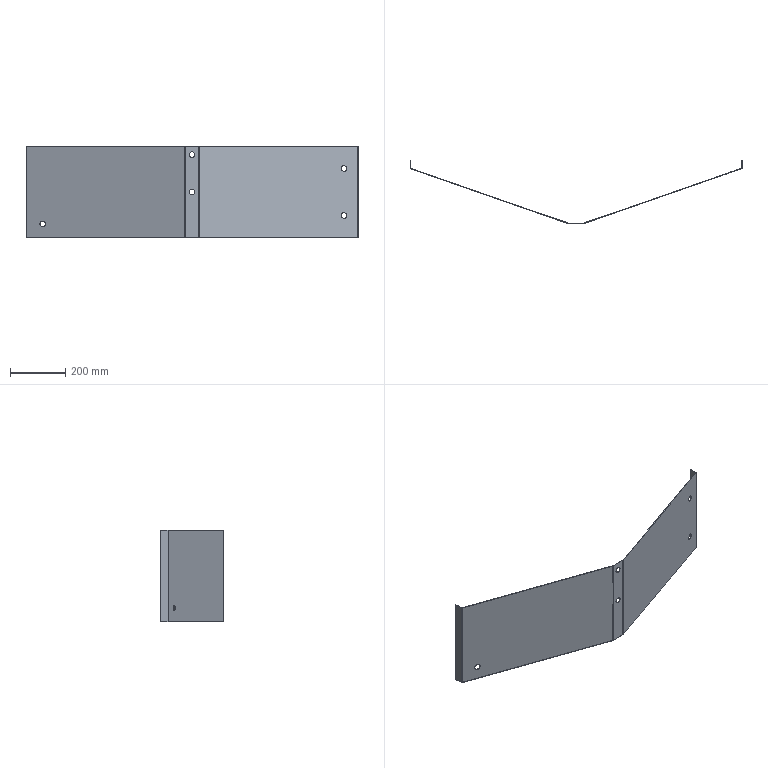Part | SolidWorks | features ICE 4, FlatPattern 1, SMBaseFlange 1, SheetMetal 1 | 1 solid | 48 faces | box 1200 x 230 x 330 mm | volume 522694 mm3 | plane 30 | cylinder 18 | commonest cylinder face diameters 20 x10 2 x4 4.4 x4
STEP:
#1=CARTESIAN_POINT('',(60.329,-19.714,40.));
#2=VERTEX_POINT('',#1);
#3=CARTESIAN_POINT('',(60.329,-19.714,60.));
#4=VERTEX_POINT('',#3);
#5=CARTESIAN_POINT('',(60.329,-19.714,40.));
#6=CARTESIAN_POINT('',(40.329,-12.757,40.));
#7=CARTESIAN_POINT('',(40.329,-12.757,60.));
#8=CARTESIAN_POINT('',(60.329,-19.714,60.));
#9=(BOUNDED_CURVE()B_SPLINE_CURVE(3,(#5,#6,#7,#8),.UNSPECIFIED.,.F.,.F.)B_SPLINE_CURVE_WITH_KNOTS((4,4),(1.571,4.712),.UNSPECIFIED.)CURVE()GEOMETRIC_REPRESENTATION_ITEM()RATIONAL_B_SPLINE_CURVE((1.,0.3333,0.3333,1.))REPRESENTATION_ITEM(''));
#10=EDGE_CURVE('',#2,#4,#9,.T.);
#11=ORIENTED_EDGE('',*,*,#10,.T.);
#12=CARTESIAN_POINT('',(60.329,-20.984,60.));
#13=VERTEX_POINT('',#12);
#14=CARTESIAN_POINT('',(60.329,30.,60.));
#15=DIRECTION('',(0.,-1.,0.));
#16=VECTOR('',#15,1000.);
#17=LINE('',#14,#16);
#18=EDGE_CURVE('',#4,#13,#17,.T.);
#19=ORIENTED_EDGE('',*,*,#18,.T.);
#20=CARTESIAN_POINT('',(60.329,-20.984,40.));
#21=VERTEX_POINT('',#20);
#22=CARTESIAN_POINT('',(60.329,-20.984,40.));
#23=CARTESIAN_POINT('',(40.329,-14.028,40.));
#24=CARTESIAN_POINT('',(40.329,-14.028,60.));
#25=CARTESIAN_POINT('',(60.329,-20.984,60.));
#26=(BOUNDED_CURVE()B_SPLINE_CURVE(3,(#22,#23,#24,#25),.UNSPECIFIED.,.F.,.F.)B_SPLINE_CURVE_WITH_KNOTS((4,4),(1.571,4.712),.UNSPECIFIED.)CURVE()GEOMETRIC_REPRESENTATION_ITEM()RATIONAL_B_SPLINE_CURVE((1.,0.3333,0.3333,1.))REPRESENTATION_ITEM(''));
#27=EDGE_CURVE('',#21,#13,#26,.T.);
#28=ORIENTED_EDGE('',*,*,#27,.F.);
#29=CARTESIAN_POINT('',(60.329,30.,40.));
#30=DIRECTION('',(0.,-1.,0.));
#31=VECTOR('',#30,1000.);
#32=LINE('',#29,#31);
#33=EDGE_CURVE('',#2,#21,#32,.T.);
#34=ORIENTED_EDGE('',*,*,#33,.F.);
#35=EDGE_LOOP('',(#11,#19,#28,#34));
#36=FACE_OUTER_BOUND('',#35,.T.);
#37=CARTESIAN_POINT('',(60.329,30.,50.));
#38=DIRECTION('',(0.,-1.,0.));
#39=DIRECTION('',(0.,0.,-1.));
#40=AXIS2_PLACEMENT_3D('',#37,#38,#39);
#41=CYLINDRICAL_SURFACE('',#40,10.);
#42=ADVANCED_FACE('',(#36),#41,.F.);
#43=CARTESIAN_POINT('',(1149.665,-16.237,240.));
#44=VERTEX_POINT('',#43);
#45=CARTESIAN_POINT('',(1149.665,-16.237,260.));
#46=VERTEX_POINT('',#45);
#47=CARTESIAN_POINT('',(1149.665,-16.237,240.));
#48=CARTESIAN_POINT('',(1129.665,-23.194,240.));
#49=CARTESIAN_POINT('',(1129.665,-23.194,260.));
#50=CARTESIAN_POINT('',(1149.665,-16.237,260.));
#51=(BOUNDED_CURVE()B_SPLINE_CURVE(3,(#47,#48,#49,#50),.UNSPECIFIED.,.F.,.F.)B_SPLINE_CURVE_WITH_KNOTS((4,4),(4.712,7.854),.UNSPECIFIED.)CURVE()GEOMETRIC_REPRESENTATION_ITEM()RATIONAL_B_SPLINE_CURVE((1.,0.3333,0.3333,1.))REPRESENTATION_ITEM(''));
#52=EDGE_CURVE('',#44,#46,#51,.T.);
#53=ORIENTED_EDGE('',*,*,#52,.T.);
#54=CARTESIAN_POINT('',(1149.665,-17.508,260.));
#55=VERTEX_POINT('',#54);
#56=CARTESIAN_POINT('',(1149.665,30.,260.));
#57=DIRECTION('',(0.,-1.,0.));
#58=VECTOR('',#57,1000.);
#59=LINE('',#56,#58);
#60=EDGE_CURVE('',#46,#55,#59,.T.);
#61=ORIENTED_EDGE('',*,*,#60,.T.);
#62=CARTESIAN_POINT('',(1149.665,-17.508,240.));
#63=VERTEX_POINT('',#62);
#64=CARTESIAN_POINT('',(1149.665,-17.508,240.));
#65=CARTESIAN_POINT('',(1129.665,-24.464,240.));
#66=CARTESIAN_POINT('',(1129.665,-24.464,260.));
#67=CARTESIAN_POINT('',(1149.665,-17.508,260.));
#68=(BOUNDED_CURVE()B_SPLINE_CURVE(3,(#64,#65,#66,#67),.UNSPECIFIED.,.F.,.F.)B_SPLINE_CURVE_WITH_KNOTS((4,4),(4.712,7.854),.UNSPECIFIED.)CURVE()GEOMETRIC_REPRESENTATION_ITEM()RATIONAL_B_SPLINE_CURVE((1.,0.3333,0.3333,1.))REPRESENTATION_ITEM(''));
#69=EDGE_CURVE('',#63,#55,#68,.T.);
#70=ORIENTED_EDGE('',*,*,#69,.F.);
#71=CARTESIAN_POINT('',(1149.665,30.,240.));
#72=DIRECTION('',(0.,-1.,0.));
#73=VECTOR('',#72,1000.);
#74=LINE('',#71,#73);
#75=EDGE_CURVE('',#44,#63,#74,.T.);
#76=ORIENTED_EDGE('',*,*,#75,.F.);
#77=EDGE_LOOP('',(#53,#61,#70,#76));
#78=FACE_OUTER_BOUND('',#77,.T.);
#79=CARTESIAN_POINT('',(1149.665,30.,250.));
#80=DIRECTION('',(0.,-1.,0.));
#81=DIRECTION('',(0.,0.,-1.));
#82=AXIS2_PLACEMENT_3D('',#79,#80,#81);
#83=CYLINDRICAL_SURFACE('',#82,10.);
#84=ADVANCED_FACE('',(#78),#83,.F.);
#85=CARTESIAN_POINT('',(1149.665,-16.237,70.));
#86=VERTEX_POINT('',#85);
#87=CARTESIAN_POINT('',(1149.665,-16.237,90.));
#88=VERTEX_POINT('',#87);
#89=CARTESIAN_POINT('',(1149.665,-16.237,70.));
#90=CARTESIAN_POINT('',(1129.665,-23.194,70.));
#91=CARTESIAN_POINT('',(1129.665,-23.194,90.));
#92=CARTESIAN_POINT('',(1149.665,-16.237,90.));
#93=(BOUNDED_CURVE()B_SPLINE_CURVE(3,(#89,#90,#91,#92),.UNSPECIFIED.,.F.,.F.)B_SPLINE_CURVE_WITH_KNOTS((4,4),(4.712,7.854),.UNSPECIFIED.)CURVE()GEOMETRIC_REPRESENTATION_ITEM()RATIONAL_B_SPLINE_CURVE((1.,0.3333,0.3333,1.))REPRESENTATION_ITEM(''));
#94=EDGE_CURVE('',#86,#88,#93,.T.);
#95=ORIENTED_EDGE('',*,*,#94,.T.);
#96=CARTESIAN_POINT('',(1149.665,-17.508,90.));
#97=VERTEX_POINT('',#96);
#98=CARTESIAN_POINT('',(1149.665,30.,90.));
#99=DIRECTION('',(0.,-1.,0.));
#100=VECTOR('',#99,1000.);
#101=LINE('',#98,#100);
#102=EDGE_CURVE('',#88,#97,#101,.T.);
#103=ORIENTED_EDGE('',*,*,#102,.T.);
#104=CARTESIAN_POINT('',(1149.665,-17.508,70.));
#105=VERTEX_POINT('',#104);
#106=CARTESIAN_POINT('',(1149.665,-17.508,70.));
#107=CARTESIAN_POINT('',(1129.665,-24.464,70.));
#108=CARTESIAN_POINT('',(1129.665,-24.464,90.));
#109=CARTESIAN_POINT('',(1149.665,-17.508,90.));
#110=(BOUNDED_CURVE()B_SPLINE_CURVE(3,(#106,#107,#108,#109),.UNSPECIFIED.,.F.,.F.)B_SPLINE_CURVE_WITH_KNOTS((4,4),(4.712,7.854),.UNSPECIFIED.)CURVE()GEOMETRIC_REPRESENTATION_ITEM()RATIONAL_B_SPLINE_CURVE((1.,0.3333,0.3333,1.))REPRESENTATION_ITEM(''));
#111=EDGE_CURVE('',#105,#97,#110,.T.);
#112=ORIENTED_EDGE('',*,*,#111,.F.);
#113=CARTESIAN_POINT('',(1149.665,30.,70.));
#114=DIRECTION('',(0.,-1.,0.));
#115=VECTOR('',#114,1000.);
#116=LINE('',#113,#115);
#117=EDGE_CURVE('',#86,#105,#116,.T.);
#118=ORIENTED_EDGE('',*,*,#117,.F.);
#119=EDGE_LOOP('',(#95,#103,#112,#118));
#120=FACE_OUTER_BOUND('',#119,.T.);
#121=CARTESIAN_POINT('',(1149.665,30.,80.));
#122=DIRECTION('',(0.,-1.,0.));
#123=DIRECTION('',(0.,0.,-1.));
#124=AXIS2_PLACEMENT_3D('',#121,#122,#123);
#125=CYLINDRICAL_SURFACE('',#124,10.);
#126=ADVANCED_FACE('',(#120),#125,.F.);
#127=CARTESIAN_POINT('',(600.,-200.,155.));
#128=VERTEX_POINT('',#127);
#129=CARTESIAN_POINT('',(600.,-200.,175.));
#130=VERTEX_POINT('',#129);
#131=CARTESIAN_POINT('',(600.,-200.,165.));
#132=DIRECTION('',(0.,1.,0.));
#133=DIRECTION('',(0.,0.,1.));
#134=AXIS2_PLACEMENT_3D('',#131,#132,#133);
#135=CIRCLE('',#134,10.);
#136=EDGE_CURVE('',#128,#130,#135,.T.);
#137=ORIENTED_EDGE('',*,*,#136,.F.);
#138=CARTESIAN_POINT('',(600.,-198.8,155.));
#139=VERTEX_POINT('',#138);
#140=CARTESIAN_POINT('',(600.,-208.8,155.));
#141=DIRECTION('',(0.,1.,0.));
#142=VECTOR('',#141,1000.);
#143=LINE('',#140,#142);
#144=EDGE_CURVE('',#128,#139,#143,.T.);
#145=ORIENTED_EDGE('',*,*,#144,.T.);
#146=CARTESIAN_POINT('',(600.,-198.8,175.));
#147=VERTEX_POINT('',#146);
#148=CARTESIAN_POINT('',(600.,-198.8,165.));
#149=DIRECTION('',(0.,1.,0.));
#150=DIRECTION('',(0.,0.,1.));
#151=AXIS2_PLACEMENT_3D('',#148,#149,#150);
#152=CIRCLE('',#151,10.);
#153=EDGE_CURVE('',#139,#147,#152,.T.);
#154=ORIENTED_EDGE('',*,*,#153,.T.);
#155=CARTESIAN_POINT('',(600.,-208.8,175.));
#156=DIRECTION('',(0.,1.,0.));
#157=VECTOR('',#156,1000.);
#158=LINE('',#155,#157);
#159=EDGE_CURVE('',#130,#147,#158,.T.);
#160=ORIENTED_EDGE('',*,*,#159,.F.);
#161=EDGE_LOOP('',(#137,#145,#154,#160));
#162=FACE_OUTER_BOUND('',#161,.T.);
#163=CARTESIAN_POINT('',(600.,-208.8,165.));
#164=DIRECTION('',(0.,1.,0.));
#165=DIRECTION('',(0.,0.,1.));
#166=AXIS2_PLACEMENT_3D('',#163,#164,#165);
#167=CYLINDRICAL_SURFACE('',#166,10.);
#168=ADVANCED_FACE('',(#162),#167,.F.);
#169=CARTESIAN_POINT('',(600.,-200.,290.));
#170=VERTEX_POINT('',#169);
#171=CARTESIAN_POINT('',(600.,-200.,310.));
#172=VERTEX_POINT('',#171);
#173=CARTESIAN_POINT('',(600.,-200.,300.));
#174=DIRECTION('',(0.,1.,0.));
#175=DIRECTION('',(0.,0.,1.));
#176=AXIS2_PLACEMENT_3D('',#173,#174,#175);
#177=CIRCLE('',#176,10.);
#178=EDGE_CURVE('',#170,#172,#177,.T.);
#179=ORIENTED_EDGE('',*,*,#178,.F.);
#180=CARTESIAN_POINT('',(600.,-198.8,290.));
#181=VERTEX_POINT('',#180);
#182=CARTESIAN_POINT('',(600.,-208.8,290.));
#183=DIRECTION('',(0.,1.,0.));
#184=VECTOR('',#183,1000.);
#185=LINE('',#182,#184);
#186=EDGE_CURVE('',#170,#181,#185,.T.);
#187=ORIENTED_EDGE('',*,*,#186,.T.);
#188=CARTESIAN_POINT('',(600.,-198.8,310.));
#189=VERTEX_POINT('',#188);
#190=CARTESIAN_POINT('',(600.,-198.8,300.));
#191=DIRECTION('',(0.,1.,0.));
#192=DIRECTION('',(0.,0.,1.));
#193=AXIS2_PLACEMENT_3D('',#190,#191,#192);
#194=CIRCLE('',#193,10.);
#195=EDGE_CURVE('',#181,#189,#194,.T.);
#196=ORIENTED_EDGE('',*,*,#195,.T.);
#197=CARTESIAN_POINT('',(600.,-208.8,310.));
#198=DIRECTION('',(0.,1.,0.));
#199=VECTOR('',#198,1000.);
#200=LINE('',#197,#199);
#201=EDGE_CURVE('',#172,#189,#200,.T.);
#202=ORIENTED_EDGE('',*,*,#201,.F.);
#203=EDGE_LOOP('',(#179,#187,#196,#202));
#204=FACE_OUTER_BOUND('',#203,.T.);
#205=CARTESIAN_POINT('',(600.,-208.8,300.));
#206=DIRECTION('',(0.,1.,0.));
#207=DIRECTION('',(0.,0.,1.));
#208=AXIS2_PLACEMENT_3D('',#205,#206,#207);
#209=CYLINDRICAL_SURFACE('',#208,10.);
#210=ADVANCED_FACE('',(#204),#209,.F.);
#211=CARTESIAN_POINT('',(0.,1.564,330.));
#212=VERTEX_POINT('',#211);
#213=CARTESIAN_POINT('',(1.2,1.564,330.));
#214=VERTEX_POINT('',#213);
#215=CARTESIAN_POINT('',(0.,1.564,330.));
#216=DIRECTION('',(1.,0.,0.));
#217=VECTOR('',#216,1000.);
#218=LINE('',#215,#217);
#219=EDGE_CURVE('',#212,#214,#218,.T.);
#220=ORIENTED_EDGE('',*,*,#219,.F.);
#221=CARTESIAN_POINT('',(1.477,-0.5138,330.));
#222=VERTEX_POINT('',#221);
#223=CARTESIAN_POINT('',(2.2,1.564,330.));
#224=DIRECTION('',(0.,0.,1.));
#225=DIRECTION('',(-1.,0.,0.));
#226=AXIS2_PLACEMENT_3D('',#223,#224,#225);
#227=CIRCLE('',#226,2.2);
#228=EDGE_CURVE('',#212,#222,#227,.T.);
#229=ORIENTED_EDGE('',*,*,#228,.T.);
#230=CARTESIAN_POINT('',(1.871,0.6196,330.));
#231=VERTEX_POINT('',#230);
#232=CARTESIAN_POINT('',(1.871,0.6196,330.));
#233=DIRECTION('',(-0.3285,-0.9445,0.));
#234=VECTOR('',#233,1000.);
#235=LINE('',#232,#234);
#236=EDGE_CURVE('',#231,#222,#235,.T.);
#237=ORIENTED_EDGE('',*,*,#236,.F.);
#238=CARTESIAN_POINT('',(2.2,1.564,330.));
#239=DIRECTION('',(0.,0.,1.));
#240=DIRECTION('',(1.,0.,0.));
#241=AXIS2_PLACEMENT_3D('',#238,#239,#240);
#242=CIRCLE('',#241,1.);
#243=EDGE_CURVE('',#214,#231,#242,.T.);
#244=ORIENTED_EDGE('',*,*,#243,.F.);
#245=EDGE_LOOP('',(#220,#229,#237,#244));
#246=FACE_OUTER_BOUND('',#245,.T.);
#247=CARTESIAN_POINT('',(0.,1.564,330.));
#248=DIRECTION('',(0.,0.,1.));
#249=DIRECTION('',(1.,0.,0.));
#250=AXIS2_PLACEMENT_3D('',#247,#248,#249);
#251=PLANE('',#250);
#252=ADVANCED_FACE('',(#246),#251,.T.);
#253=CARTESIAN_POINT('',(0.,30.,330.));
#254=VERTEX_POINT('',#253);
#255=CARTESIAN_POINT('',(0.,0.,330.));
#256=DIRECTION('',(0.,-1.,0.));
#257=VECTOR('',#256,1000.);
#258=LINE('',#255,#257);
#259=EDGE_CURVE('',#254,#212,#258,.T.);
#260=ORIENTED_EDGE('',*,*,#259,.T.);
#261=ORIENTED_EDGE('',*,*,#219,.T.);
#262=CARTESIAN_POINT('',(1.2,30.,330.));
#263=VERTEX_POINT('',#262);
#264=CARTESIAN_POINT('',(1.2,0.,330.));
#265=DIRECTION('',(0.,-1.,0.));
#266=VECTOR('',#265,1000.);
#267=LINE('',#264,#266);
#268=EDGE_CURVE('',#263,#214,#267,.T.);
#269=ORIENTED_EDGE('',*,*,#268,.F.);
#270=CARTESIAN_POINT('',(0.,30.,330.));
#271=DIRECTION('',(1.,0.,0.));
#272=VECTOR('',#271,1000.);
#273=LINE('',#270,#272);
#274=EDGE_CURVE('',#254,#263,#273,.T.);
#275=ORIENTED_EDGE('',*,*,#274,.F.);
#276=EDGE_LOOP('',(#260,#261,#269,#275));
#277=FACE_OUTER_BOUND('',#276,.T.);
#278=CARTESIAN_POINT('',(1.871,0.6196,330.));
#279=DIRECTION('',(0.,0.,1.));
#280=DIRECTION('',(1.,0.,0.));
#281=AXIS2_PLACEMENT_3D('',#278,#279,#280);
#282=PLANE('',#281);
#283=ADVANCED_FACE('',(#277),#282,.T.);
#284=CARTESIAN_POINT('',(1.477,-0.5138,0.));
#285=VERTEX_POINT('',#284);
#286=CARTESIAN_POINT('',(1.871,0.6196,0.));
#287=VERTEX_POINT('',#286);
#288=CARTESIAN_POINT('',(1.477,-0.5138,0.));
#289=DIRECTION('',(0.3285,0.9445,0.));
#290=VECTOR('',#289,1000.);
#291=LINE('',#288,#290);
#292=EDGE_CURVE('',#285,#287,#291,.T.);
#293=ORIENTED_EDGE('',*,*,#292,.F.);
#294=CARTESIAN_POINT('',(0.,1.564,0.));
#295=VERTEX_POINT('',#294);
#296=CARTESIAN_POINT('',(2.2,1.564,0.));
#297=DIRECTION('',(0.,0.,1.));
#298=DIRECTION('',(-1.,0.,0.));
#299=AXIS2_PLACEMENT_3D('',#296,#297,#298);
#300=CIRCLE('',#299,2.2);
#301=EDGE_CURVE('',#295,#285,#300,.T.);
#302=ORIENTED_EDGE('',*,*,#301,.F.);
#303=CARTESIAN_POINT('',(1.2,1.564,0.));
#304=VERTEX_POINT('',#303);
#305=CARTESIAN_POINT('',(1.2,1.564,0.));
#306=DIRECTION('',(-1.,0.,0.));
#307=VECTOR('',#306,1000.);
#308=LINE('',#305,#307);
#309=EDGE_CURVE('',#304,#295,#308,.T.);
#310=ORIENTED_EDGE('',*,*,#309,.F.);
#311=CARTESIAN_POINT('',(2.2,1.564,0.));
#312=DIRECTION('',(0.,0.,1.));
#313=DIRECTION('',(1.,0.,0.));
#314=AXIS2_PLACEMENT_3D('',#311,#312,#313);
#315=CIRCLE('',#314,1.);
#316=EDGE_CURVE('',#304,#287,#315,.T.);
#317=ORIENTED_EDGE('',*,*,#316,.T.);
#318=EDGE_LOOP('',(#293,#302,#310,#317));
#319=FACE_OUTER_BOUND('',#318,.T.);
#320=CARTESIAN_POINT('',(1.477,-0.5138,0.));
#321=DIRECTION('',(0.,0.,-1.));
#322=DIRECTION('',(-1.,0.,0.));
#323=AXIS2_PLACEMENT_3D('',#320,#321,#322);
#324=PLANE('',#323);
#325=ADVANCED_FACE('',(#319),#324,.T.);
#326=CARTESIAN_POINT('',(574.649,-199.878,0.));
#327=VERTEX_POINT('',#326);
#328=CARTESIAN_POINT('',(0.,0.,0.));
#329=DIRECTION('',(0.9445,-0.3285,0.));
#330=VECTOR('',#329,1000.);
#331=LINE('',#328,#330);
#332=EDGE_CURVE('',#285,#327,#331,.T.);
#333=ORIENTED_EDGE('',*,*,#332,.F.);
#334=ORIENTED_EDGE('',*,*,#292,.T.);
#335=CARTESIAN_POINT('',(575.043,-198.744,0.));
#336=VERTEX_POINT('',#335);
#337=CARTESIAN_POINT('',(0.3942,1.133,0.));
#338=DIRECTION('',(0.9445,-0.3285,0.));
#339=VECTOR('',#338,1000.);
#340=LINE('',#337,#339);
#341=EDGE_CURVE('',#287,#336,#340,.T.);
#342=ORIENTED_EDGE('',*,*,#341,.T.);
#343=CARTESIAN_POINT('',(575.043,-198.744,0.));
#344=DIRECTION('',(-0.3285,-0.9445,0.));
#345=VECTOR('',#344,1000.);
#346=LINE('',#343,#345);
#347=EDGE_CURVE('',#336,#327,#346,.T.);
#348=ORIENTED_EDGE('',*,*,#347,.T.);
#349=EDGE_LOOP('',(#333,#334,#342,#348));
#350=FACE_OUTER_BOUND('',#349,.T.);
#351=CARTESIAN_POINT('',(1.2,1.564,0.));
#352=DIRECTION('',(0.,0.,-1.));
#353=DIRECTION('',(-1.,0.,0.));
#354=AXIS2_PLACEMENT_3D('',#351,#352,#353);
#355=PLANE('',#354);
#356=ADVANCED_FACE('',(#350),#355,.T.);
#357=CARTESIAN_POINT('',(574.649,-199.878,330.));
#358=VERTEX_POINT('',#357);
#359=CARTESIAN_POINT('',(575.043,-198.744,330.));
#360=VERTEX_POINT('',#359);
#361=CARTESIAN_POINT('',(574.649,-199.878,330.));
#362=DIRECTION('',(0.3285,0.9445,0.));
#363=VECTOR('',#362,1000.);
#364=LINE('',#361,#363);
#365=EDGE_CURVE('',#358,#360,#364,.T.);
#366=ORIENTED_EDGE('',*,*,#365,.F.);
#367=CARTESIAN_POINT('',(575.372,-200.,330.));
#368=VERTEX_POINT('',#367);
#369=CARTESIAN_POINT('',(575.372,-197.8,330.));
#370=DIRECTION('',(0.,0.,1.));
#371=DIRECTION('',(-1.,0.,0.));
#372=AXIS2_PLACEMENT_3D('',#369,#370,#371);
#373=CIRCLE('',#372,2.2);
#374=EDGE_CURVE('',#358,#368,#373,.T.);
#375=ORIENTED_EDGE('',*,*,#374,.T.);
#376=CARTESIAN_POINT('',(575.372,-198.8,330.));
#377=VERTEX_POINT('',#376);
#378=CARTESIAN_POINT('',(575.372,-198.8,330.));
#379=DIRECTION('',(0.,-1.,0.));
#380=VECTOR('',#379,1000.);
#381=LINE('',#378,#380);
#382=EDGE_CURVE('',#377,#368,#381,.T.);
#383=ORIENTED_EDGE('',*,*,#382,.F.);
#384=CARTESIAN_POINT('',(575.372,-197.8,330.));
#385=DIRECTION('',(0.,0.,1.));
#386=DIRECTION('',(1.,0.,0.));
#387=AXIS2_PLACEMENT_3D('',#384,#385,#386);
#388=CIRCLE('',#387,1.);
#389=EDGE_CURVE('',#360,#377,#388,.T.);
#390=ORIENTED_EDGE('',*,*,#389,.F.);
#391=EDGE_LOOP('',(#366,#375,#383,#390));
#392=FACE_OUTER_BOUND('',#391,.T.);
#393=CARTESIAN_POINT('',(574.649,-199.878,330.));
#394=DIRECTION('',(0.,0.,1.));
#395=DIRECTION('',(1.,0.,0.));
#396=AXIS2_PLACEMENT_3D('',#393,#394,#395);
#397=PLANE('',#396);
#398=ADVANCED_FACE('',(#392),#397,.T.);
#399=CARTESIAN_POINT('',(0.,0.,330.));
#400=DIRECTION('',(0.9445,-0.3285,0.));
#401=VECTOR('',#400,1000.);
#402=LINE('',#399,#401);
#403=EDGE_CURVE('',#222,#358,#402,.T.);
#404=ORIENTED_EDGE('',*,*,#403,.T.);
#405=ORIENTED_EDGE('',*,*,#365,.T.);
#406=CARTESIAN_POINT('',(0.3942,1.133,330.));
#407=DIRECTION('',(0.9445,-0.3285,0.));
#408=VECTOR('',#407,1000.);
#409=LINE('',#406,#408);
#410=EDGE_CURVE('',#231,#360,#409,.T.);
#411=ORIENTED_EDGE('',*,*,#410,.F.);
#412=ORIENTED_EDGE('',*,*,#236,.T.);
#413=EDGE_LOOP('',(#404,#405,#411,#412));
#414=FACE_OUTER_BOUND('',#413,.T.);
#415=CARTESIAN_POINT('',(575.372,-198.8,330.));
#416=DIRECTION('',(0.,0.,1.));
#417=DIRECTION('',(1.,0.,0.));
#418=AXIS2_PLACEMENT_3D('',#415,#416,#417);
#419=PLANE('',#418);
#420=ADVANCED_FACE('',(#414),#419,.T.);
#421=CARTESIAN_POINT('',(575.372,-200.,0.));
#422=VERTEX_POINT('',#421);
#423=CARTESIAN_POINT('',(575.372,-198.8,0.));
#424=VERTEX_POINT('',#423);
#425=CARTESIAN_POINT('',(575.372,-200.,0.));
#426=DIRECTION('',(0.,1.,0.));
#427=VECTOR('',#426,1000.);
#428=LINE('',#425,#427);
#429=EDGE_CURVE('',#422,#424,#428,.T.);
#430=ORIENTED_EDGE('',*,*,#429,.F.);
#431=CARTESIAN_POINT('',(575.372,-197.8,0.));
#432=DIRECTION('',(0.,0.,1.));
#433=DIRECTION('',(-1.,0.,0.));
#434=AXIS2_PLACEMENT_3D('',#431,#432,#433);
#435=CIRCLE('',#434,2.2);
#436=EDGE_CURVE('',#327,#422,#435,.T.);
#437=ORIENTED_EDGE('',*,*,#436,.F.);
#438=ORIENTED_EDGE('',*,*,#347,.F.);
#439=CARTESIAN_POINT('',(575.372,-197.8,0.));
#440=DIRECTION('',(0.,0.,1.));
#441=DIRECTION('',(1.,0.,0.));
#442=AXIS2_PLACEMENT_3D('',#439,#440,#441);
#443=CIRCLE('',#442,1.);
#444=EDGE_CURVE('',#336,#424,#443,.T.);
#445=ORIENTED_EDGE('',*,*,#444,.T.);
#446=EDGE_LOOP('',(#430,#437,#438,#445));
#447=FACE_OUTER_BOUND('',#446,.T.);
#448=CARTESIAN_POINT('',(575.372,-200.,0.));
#449=DIRECTION('',(0.,0.,-1.));
#450=DIRECTION('',(-1.,0.,0.));
#451=AXIS2_PLACEMENT_3D('',#448,#449,#450);
#452=PLANE('',#451);
#453=ADVANCED_FACE('',(#447),#452,.T.);
#454=CARTESIAN_POINT('',(624.628,-200.,0.));
#455=VERTEX_POINT('',#454);
#456=CARTESIAN_POINT('',(575.,-200.,0.));
#457=DIRECTION('',(1.,0.,0.));
#458=VECTOR('',#457,1000.);
#459=LINE('',#456,#458);
#460=EDGE_CURVE('',#422,#455,#459,.T.);
#461=ORIENTED_EDGE('',*,*,#460,.F.);
#462=ORIENTED_EDGE('',*,*,#429,.T.);
#463=CARTESIAN_POINT('',(624.628,-198.8,0.));
#464=VERTEX_POINT('',#463);
#465=CARTESIAN_POINT('',(575.,-198.8,0.));
#466=DIRECTION('',(1.,0.,0.));
#467=VECTOR('',#466,1000.);
#468=LINE('',#465,#467);
#469=EDGE_CURVE('',#424,#464,#468,.T.);
#470=ORIENTED_EDGE('',*,*,#469,.T.);
#471=CARTESIAN_POINT('',(624.628,-198.8,0.));
#472=DIRECTION('',(0.,-1.,0.));
#473=VECTOR('',#472,1000.);
#474=LINE('',#471,#473);
#475=EDGE_CURVE('',#464,#455,#474,.T.);
#476=ORIENTED_EDGE('',*,*,#475,.T.);
#477=EDGE_LOOP('',(#461,#462,#470,#476));
#478=FACE_OUTER_BOUND('',#477,.T.);
#479=CARTESIAN_POINT('',(575.043,-198.744,0.));
#480=DIRECTION('',(0.,0.,-1.));
#481=DIRECTION('',(-1.,0.,0.));
#482=AXIS2_PLACEMENT_3D('',#479,#480,#481);
#483=PLANE('',#482);
#484=ADVANCED_FACE('',(#478),#483,.T.);
#485=CARTESIAN_POINT('',(624.628,-200.,330.));
#486=VERTEX_POINT('',#485);
#487=CARTESIAN_POINT('',(624.628,-198.8,330.));
#488=VERTEX_POINT('',#487);
#489=CARTESIAN_POINT('',(624.628,-200.,330.));
#490=DIRECTION('',(0.,1.,0.));
#491=VECTOR('',#490,1000.);
#492=LINE('',#489,#491);
#493=EDGE_CURVE('',#486,#488,#492,.T.);
#494=ORIENTED_EDGE('',*,*,#493,.F.);
#495=CARTESIAN_POINT('',(625.351,-199.878,330.));
#496=VERTEX_POINT('',#495);
#497=CARTESIAN_POINT('',(624.628,-197.8,330.));
#498=DIRECTION('',(0.,0.,1.));
#499=DIRECTION('',(-1.,0.,0.));
#500=AXIS2_PLACEMENT_3D('',#497,#498,#499);
#501=CIRCLE('',#500,2.2);
#502=EDGE_CURVE('',#486,#496,#501,.T.);
#503=ORIENTED_EDGE('',*,*,#502,.T.);
#504=CARTESIAN_POINT('',(624.957,-198.744,330.));
#505=VERTEX_POINT('',#504);
#506=CARTESIAN_POINT('',(624.957,-198.744,330.));
#507=DIRECTION('',(0.3285,-0.9445,0.));
#508=VECTOR('',#507,1000.);
#509=LINE('',#506,#508);
#510=EDGE_CURVE('',#505,#496,#509,.T.);
#511=ORIENTED_EDGE('',*,*,#510,.F.);
#512=CARTESIAN_POINT('',(624.628,-197.8,330.));
#513=DIRECTION('',(0.,0.,1.));
#514=DIRECTION('',(1.,0.,0.));
#515=AXIS2_PLACEMENT_3D('',#512,#513,#514);
#516=CIRCLE('',#515,1.);
#517=EDGE_CURVE('',#488,#505,#516,.T.);
#518=ORIENTED_EDGE('',*,*,#517,.F.);
#519=EDGE_LOOP('',(#494,#503,#511,#518));
#520=FACE_OUTER_BOUND('',#519,.T.);
#521=CARTESIAN_POINT('',(624.628,-200.,330.));
#522=DIRECTION('',(0.,0.,1.));
#523=DIRECTION('',(1.,0.,0.));
#524=AXIS2_PLACEMENT_3D('',#521,#522,#523);
#525=PLANE('',#524);
#526=ADVANCED_FACE('',(#520),#525,.T.);
#527=CARTESIAN_POINT('',(575.,-200.,330.));
#528=DIRECTION('',(1.,0.,0.));
#529=VECTOR('',#528,1000.);
#530=LINE('',#527,#529);
#531=EDGE_CURVE('',#368,#486,#530,.T.);
#532=ORIENTED_EDGE('',*,*,#531,.T.);
#533=ORIENTED_EDGE('',*,*,#493,.T.);
#534=CARTESIAN_POINT('',(575.,-198.8,330.));
#535=DIRECTION('',(1.,0.,0.));
#536=VECTOR('',#535,1000.);
#537=LINE('',#534,#536);
#538=EDGE_CURVE('',#377,#488,#537,.T.);
#539=ORIENTED_EDGE('',*,*,#538,.F.);
#540=ORIENTED_EDGE('',*,*,#382,.T.);
#541=EDGE_LOOP('',(#532,#533,#539,#540));
#542=FACE_OUTER_BOUND('',#541,.T.);
#543=CARTESIAN_POINT('',(624.957,-198.744,330.));
#544=DIRECTION('',(0.,0.,1.));
#545=DIRECTION('',(1.,0.,0.));
#546=AXIS2_PLACEMENT_3D('',#543,#544,#545);
#547=PLANE('',#546);
#548=ADVANCED_FACE('',(#542),#547,.T.);
#549=CARTESIAN_POINT('',(625.351,-199.878,0.));
#550=VERTEX_POINT('',#549);
#551=CARTESIAN_POINT('',(624.957,-198.744,0.));
#552=VERTEX_POINT('',#551);
#553=CARTESIAN_POINT('',(625.351,-199.878,0.));
#554=DIRECTION('',(-0.3285,0.9445,0.));
#555=VECTOR('',#554,1000.);
#556=LINE('',#553,#555);
#557=EDGE_CURVE('',#550,#552,#556,.T.);
#558=ORIENTED_EDGE('',*,*,#557,.F.);
#559=CARTESIAN_POINT('',(624.628,-197.8,0.));
#560=DIRECTION('',(0.,0.,1.));
#561=DIRECTION('',(-1.,0.,0.));
#562=AXIS2_PLACEMENT_3D('',#559,#560,#561);
#563=CIRCLE('',#562,2.2);
#564=EDGE_CURVE('',#455,#550,#563,.T.);
#565=ORIENTED_EDGE('',*,*,#564,.F.);
#566=ORIENTED_EDGE('',*,*,#475,.F.);
#567=CARTESIAN_POINT('',(624.628,-197.8,0.));
#568=DIRECTION('',(0.,0.,1.));
#569=DIRECTION('',(1.,0.,0.));
#570=AXIS2_PLACEMENT_3D('',#567,#568,#569);
#571=CIRCLE('',#570,1.);
#572=EDGE_CURVE('',#464,#552,#571,.T.);
#573=ORIENTED_EDGE('',*,*,#572,.T.);
#574=EDGE_LOOP('',(#558,#565,#566,#573));
#575=FACE_OUTER_BOUND('',#574,.T.);
#576=CARTESIAN_POINT('',(625.351,-199.878,0.));
#577=DIRECTION('',(0.,0.,-1.));
#578=DIRECTION('',(-1.,0.,0.));
#579=AXIS2_PLACEMENT_3D('',#576,#577,#578);
#580=PLANE('',#579);
#581=ADVANCED_FACE('',(#575),#580,.T.);
#582=CARTESIAN_POINT('',(1198.523,-0.5138,0.));
#583=VERTEX_POINT('',#582);
#584=CARTESIAN_POINT('',(625.,-200.,0.));
#585=DIRECTION('',(0.9445,0.3285,0.));
#586=VECTOR('',#585,1000.);
#587=LINE('',#584,#586);
#588=EDGE_CURVE('',#550,#583,#587,.T.);
#589=ORIENTED_EDGE('',*,*,#588,.F.);
#590=ORIENTED_EDGE('',*,*,#557,.T.);
#591=CARTESIAN_POINT('',(1198.129,0.6196,0.));
#592=VERTEX_POINT('',#591);
#593=CARTESIAN_POINT('',(624.606,-198.867,0.));
#594=DIRECTION('',(0.9445,0.3285,0.));
#595=VECTOR('',#594,1000.);
#596=LINE('',#593,#595);
#597=EDGE_CURVE('',#552,#592,#596,.T.);
#598=ORIENTED_EDGE('',*,*,#597,.T.);
#599=CARTESIAN_POINT('',(1198.129,0.6196,0.));
#600=DIRECTION('',(0.3285,-0.9445,0.));
#601=VECTOR('',#600,1000.);
#602=LINE('',#599,#601);
#603=EDGE_CURVE('',#592,#583,#602,.T.);
#604=ORIENTED_EDGE('',*,*,#603,.T.);
#605=EDGE_LOOP('',(#589,#590,#598,#604));
#606=FACE_OUTER_BOUND('',#605,.T.);
#607=CARTESIAN_POINT('',(624.628,-198.8,0.));
#608=DIRECTION('',(0.,0.,-1.));
#609=DIRECTION('',(-1.,0.,0.));
#610=AXIS2_PLACEMENT_3D('',#607,#608,#609);
#611=PLANE('',#610);
#612=ADVANCED_FACE('',(#606),#611,.T.);
#613=CARTESIAN_POINT('',(1198.523,-0.5138,330.));
#614=VERTEX_POINT('',#613);
#615=CARTESIAN_POINT('',(1198.129,0.6196,330.));
#616=VERTEX_POINT('',#615);
#617=CARTESIAN_POINT('',(1198.523,-0.5138,330.));
#618=DIRECTION('',(-0.3285,0.9445,0.));
#619=VECTOR('',#618,1000.);
#620=LINE('',#617,#619);
#621=EDGE_CURVE('',#614,#616,#620,.T.);
#622=ORIENTED_EDGE('',*,*,#621,.F.);
#623=CARTESIAN_POINT('',(1200.,1.564,330.));
#624=VERTEX_POINT('',#623);
#625=CARTESIAN_POINT('',(1197.8,1.564,330.));
#626=DIRECTION('',(0.,0.,1.));
#627=DIRECTION('',(-1.,0.,0.));
#628=AXIS2_PLACEMENT_3D('',#625,#626,#627);
#629=CIRCLE('',#628,2.2);
#630=EDGE_CURVE('',#614,#624,#629,.T.);
#631=ORIENTED_EDGE('',*,*,#630,.T.);
#632=CARTESIAN_POINT('',(1198.8,1.564,330.));
#633=VERTEX_POINT('',#632);
#634=CARTESIAN_POINT('',(1198.8,1.564,330.));
#635=DIRECTION('',(1.,0.,0.));
#636=VECTOR('',#635,1000.);
#637=LINE('',#634,#636);
#638=EDGE_CURVE('',#633,#624,#637,.T.);
#639=ORIENTED_EDGE('',*,*,#638,.F.);
#640=CARTESIAN_POINT('',(1197.8,1.564,330.));
#641=DIRECTION('',(0.,0.,1.));
#642=DIRECTION('',(1.,0.,0.));
#643=AXIS2_PLACEMENT_3D('',#640,#641,#642);
#644=CIRCLE('',#643,1.);
#645=EDGE_CURVE('',#616,#633,#644,.T.);
#646=ORIENTED_EDGE('',*,*,#645,.F.);
#647=EDGE_LOOP('',(#622,#631,#639,#646));
#648=FACE_OUTER_BOUND('',#647,.T.);
#649=CARTESIAN_POINT('',(1198.523,-0.5138,330.));
#650=DIRECTION('',(0.,0.,1.));
#651=DIRECTION('',(1.,0.,0.));
#652=AXIS2_PLACEMENT_3D('',#649,#650,#651);
#653=PLANE('',#652);
#654=ADVANCED_FACE('',(#648),#653,.T.);
#655=CARTESIAN_POINT('',(625.,-200.,330.));
#656=DIRECTION('',(0.9445,0.3285,0.));
#657=VECTOR('',#656,1000.);
#658=LINE('',#655,#657);
#659=EDGE_CURVE('',#496,#614,#658,.T.);
#660=ORIENTED_EDGE('',*,*,#659,.T.);
#661=ORIENTED_EDGE('',*,*,#621,.T.);
#662=CARTESIAN_POINT('',(624.606,-198.867,330.));
#663=DIRECTION('',(0.9445,0.3285,0.));
#664=VECTOR('',#663,1000.);
#665=LINE('',#662,#664);
#666=EDGE_CURVE('',#505,#616,#665,.T.);
#667=ORIENTED_EDGE('',*,*,#666,.F.);
#668=ORIENTED_EDGE('',*,*,#510,.T.);
#669=EDGE_LOOP('',(#660,#661,#667,#668));
#670=FACE_OUTER_BOUND('',#669,.T.);
#671=CARTESIAN_POINT('',(1198.8,1.564,330.));
#672=DIRECTION('',(0.,0.,1.));
#673=DIRECTION('',(1.,0.,0.));
#674=AXIS2_PLACEMENT_3D('',#671,#672,#673);
#675=PLANE('',#674);
#676=ADVANCED_FACE('',(#670),#675,.T.);
#677=CARTESIAN_POINT('',(1200.,1.564,0.));
#678=VERTEX_POINT('',#677);
#679=CARTESIAN_POINT('',(1198.8,1.564,0.));
#680=VERTEX_POINT('',#679);
#681=CARTESIAN_POINT('',(1200.,1.564,0.));
#682=DIRECTION('',(-1.,0.,0.));
#683=VECTOR('',#682,1000.);
#684=LINE('',#681,#683);
#685=EDGE_CURVE('',#678,#680,#684,.T.);
#686=ORIENTED_EDGE('',*,*,#685,.F.);
#687=CARTESIAN_POINT('',(1197.8,1.564,0.));
#688=DIRECTION('',(0.,0.,1.));
#689=DIRECTION('',(-1.,0.,0.));
#690=AXIS2_PLACEMENT_3D('',#687,#688,#689);
#691=CIRCLE('',#690,2.2);
#692=EDGE_CURVE('',#583,#678,#691,.T.);
#693=ORIENTED_EDGE('',*,*,#692,.F.);
#694=ORIENTED_EDGE('',*,*,#603,.F.);
#695=CARTESIAN_POINT('',(1197.8,1.564,0.));
#696=DIRECTION('',(0.,0.,1.));
#697=DIRECTION('',(1.,0.,0.));
#698=AXIS2_PLACEMENT_3D('',#695,#696,#697);
#699=CIRCLE('',#698,1.);
#700=EDGE_CURVE('',#592,#680,#699,.T.);
#701=ORIENTED_EDGE('',*,*,#700,.T.);
#702=EDGE_LOOP('',(#686,#693,#694,#701));
#703=FACE_OUTER_BOUND('',#702,.T.);
#704=CARTESIAN_POINT('',(1200.,1.564,0.));
#705=DIRECTION('',(0.,0.,-1.));
#706=DIRECTION('',(-1.,0.,0.));
#707=AXIS2_PLACEMENT_3D('',#704,#705,#706);
#708=PLANE('',#707);
#709=ADVANCED_FACE('',(#703),#708,.T.);
#710=CARTESIAN_POINT('',(1200.,30.,0.));
#711=VERTEX_POINT('',#710);
#712=CARTESIAN_POINT('',(1200.,0.,0.));
#713=DIRECTION('',(0.,1.,0.));
#714=VECTOR('',#713,1000.);
#715=LINE('',#712,#714);
#716=EDGE_CURVE('',#678,#711,#715,.T.);
#717=ORIENTED_EDGE('',*,*,#716,.F.);
#718=ORIENTED_EDGE('',*,*,#685,.T.);
#719=CARTESIAN_POINT('',(1198.8,30.,0.));
#720=VERTEX_POINT('',#719);
#721=CARTESIAN_POINT('',(1198.8,0.,0.));
#722=DIRECTION('',(0.,1.,0.));
#723=VECTOR('',#722,1000.);
#724=LINE('',#721,#723);
#725=EDGE_CURVE('',#680,#720,#724,.T.);
#726=ORIENTED_EDGE('',*,*,#725,.T.);
#727=CARTESIAN_POINT('',(1198.8,30.,0.));
#728=DIRECTION('',(1.,0.,0.));
#729=VECTOR('',#728,1000.);
#730=LINE('',#727,#729);
#731=EDGE_CURVE('',#720,#711,#730,.T.);
#732=ORIENTED_EDGE('',*,*,#731,.T.);
#733=EDGE_LOOP('',(#717,#718,#726,#732));
#734=FACE_OUTER_BOUND('',#733,.T.);
#735=CARTESIAN_POINT('',(1198.129,0.6196,0.));
#736=DIRECTION('',(0.,0.,-1.));
#737=DIRECTION('',(-1.,0.,0.));
#738=AXIS2_PLACEMENT_3D('',#735,#736,#737);
#739=PLANE('',#738);
#740=ADVANCED_FACE('',(#734),#739,.T.);
#741=ORIENTED_EDGE('',*,*,#716,.T.);
#742=CARTESIAN_POINT('',(1200.,30.,330.));
#743=VERTEX_POINT('',#742);
#744=CARTESIAN_POINT('',(1200.,30.,330.));
#745=DIRECTION('',(0.,0.,-1.));
#746=VECTOR('',#745,1000.);
#747=LINE('',#744,#746);
#748=EDGE_CURVE('',#743,#711,#747,.T.);
#749=ORIENTED_EDGE('',*,*,#748,.F.);
#750=CARTESIAN_POINT('',(1200.,0.,330.));
#751=DIRECTION('',(0.,1.,0.));
#752=VECTOR('',#751,1000.);
#753=LINE('',#750,#752);
#754=EDGE_CURVE('',#624,#743,#753,.T.);
#755=ORIENTED_EDGE('',*,*,#754,.F.);
#756=CARTESIAN_POINT('',(1200.,1.564,330.));
#757=DIRECTION('',(0.,0.,-1.));
#758=VECTOR('',#757,1000.);
#759=LINE('',#756,#758);
#760=EDGE_CURVE('',#624,#678,#759,.T.);
#761=ORIENTED_EDGE('',*,*,#760,.T.);
#762=EDGE_LOOP('',(#741,#749,#755,#761));
#763=FACE_OUTER_BOUND('',#762,.T.);
#764=CARTESIAN_POINT('',(1200.,0.,330.));
#765=DIRECTION('',(-1.,0.,0.));
#766=DIRECTION('',(0.,0.,1.));
#767=AXIS2_PLACEMENT_3D('',#764,#765,#766);
#768=PLANE('',#767);
#769=ADVANCED_FACE('',(#763),#768,.F.);
#770=ORIENTED_EDGE('',*,*,#731,.F.);
#771=CARTESIAN_POINT('',(1198.8,30.,330.));
#772=VERTEX_POINT('',#771);
#773=CARTESIAN_POINT('',(1198.8,30.,330.));
#774=DIRECTION('',(0.,0.,-1.));
#775=VECTOR('',#774,1000.);
#776=LINE('',#773,#775);
#777=EDGE_CURVE('',#772,#720,#776,.T.);
#778=ORIENTED_EDGE('',*,*,#777,.F.);
#779=CARTESIAN_POINT('',(1198.8,30.,330.));
#780=DIRECTION('',(1.,0.,0.));
#781=VECTOR('',#780,1000.);
#782=LINE('',#779,#781);
#783=EDGE_CURVE('',#772,#743,#782,.T.);
#784=ORIENTED_EDGE('',*,*,#783,.T.);
#785=ORIENTED_EDGE('',*,*,#748,.T.);
#786=EDGE_LOOP('',(#770,#778,#784,#785));
#787=FACE_OUTER_BOUND('',#786,.T.);
#788=CARTESIAN_POINT('',(1198.8,30.,330.));
#789=DIRECTION('',(0.,1.,0.));
#790=DIRECTION('',(0.,0.,1.));
#791=AXIS2_PLACEMENT_3D('',#788,#789,#790);
#792=PLANE('',#791);
#793=ADVANCED_FACE('',(#787),#792,.T.);
#794=ORIENTED_EDGE('',*,*,#725,.F.);
#795=CARTESIAN_POINT('',(1198.8,1.564,330.));
#796=DIRECTION('',(0.,0.,-1.));
#797=VECTOR('',#796,1000.);
#798=LINE('',#795,#797);
#799=EDGE_CURVE('',#633,#680,#798,.T.);
#800=ORIENTED_EDGE('',*,*,#799,.F.);
#801=CARTESIAN_POINT('',(1198.8,0.,330.));
#802=DIRECTION('',(0.,1.,0.));
#803=VECTOR('',#802,1000.);
#804=LINE('',#801,#803);
#805=EDGE_CURVE('',#633,#772,#804,.T.);
#806=ORIENTED_EDGE('',*,*,#805,.T.);
#807=ORIENTED_EDGE('',*,*,#777,.T.);
#808=EDGE_LOOP('',(#794,#800,#806,#807));
#809=FACE_OUTER_BOUND('',#808,.T.);
#810=CARTESIAN_POINT('',(1198.8,0.,330.));
#811=DIRECTION('',(-1.,0.,0.));
#812=DIRECTION('',(0.,0.,1.));
#813=AXIS2_PLACEMENT_3D('',#810,#811,#812);
#814=PLANE('',#813);
#815=ADVANCED_FACE('',(#809),#814,.T.);
#816=ORIENTED_EDGE('',*,*,#700,.F.);
#817=CARTESIAN_POINT('',(1198.129,0.6196,330.));
#818=DIRECTION('',(0.,0.,-1.));
#819=VECTOR('',#818,1000.);
#820=LINE('',#817,#819);
#821=EDGE_CURVE('',#616,#592,#820,.T.);
#822=ORIENTED_EDGE('',*,*,#821,.F.);
#823=ORIENTED_EDGE('',*,*,#645,.T.);
#824=ORIENTED_EDGE('',*,*,#799,.T.);
#825=EDGE_LOOP('',(#816,#822,#823,#824));
#826=FACE_OUTER_BOUND('',#825,.T.);
#827=CARTESIAN_POINT('',(1197.8,1.564,330.));
#828=DIRECTION('',(0.,0.,-1.));
#829=DIRECTION('',(-1.,0.,0.));
#830=AXIS2_PLACEMENT_3D('',#827,#828,#829);
#831=CYLINDRICAL_SURFACE('',#830,1.);
#832=ADVANCED_FACE('',(#826),#831,.F.);
#833=ORIENTED_EDGE('',*,*,#52,.F.);
#834=CARTESIAN_POINT('',(1149.665,-16.237,260.));
#835=CARTESIAN_POINT('',(1169.665,-9.281,260.));
#836=CARTESIAN_POINT('',(1169.665,-9.281,240.));
#837=CARTESIAN_POINT('',(1149.665,-16.237,240.));
#838=(BOUNDED_CURVE()B_SPLINE_CURVE(3,(#834,#835,#836,#837),.UNSPECIFIED.,.F.,.T.)B_SPLINE_CURVE_WITH_KNOTS((4,4),(1.571,4.712),.UNSPECIFIED.)CURVE()GEOMETRIC_REPRESENTATION_ITEM()RATIONAL_B_SPLINE_CURVE((1.,0.3333,0.3333,1.))REPRESENTATION_ITEM(''));
#839=EDGE_CURVE('',#46,#44,#838,.T.);
#840=ORIENTED_EDGE('',*,*,#839,.F.);
#841=EDGE_LOOP('',(#833,#840));
#842=FACE_BOUND('',#841,.T.);
#843=ORIENTED_EDGE('',*,*,#94,.F.);
#844=CARTESIAN_POINT('',(1149.665,-16.237,90.));
#845=CARTESIAN_POINT('',(1169.665,-9.281,90.));
#846=CARTESIAN_POINT('',(1169.665,-9.281,70.));
#847=CARTESIAN_POINT('',(1149.665,-16.237,70.));
#848=(BOUNDED_CURVE()B_SPLINE_CURVE(3,(#844,#845,#846,#847),.UNSPECIFIED.,.F.,.F.)B_SPLINE_CURVE_WITH_KNOTS((4,4),(1.571,4.712),.UNSPECIFIED.)CURVE()GEOMETRIC_REPRESENTATION_ITEM()RATIONAL_B_SPLINE_CURVE((1.,0.3333,0.3333,1.))REPRESENTATION_ITEM(''));
#849=EDGE_CURVE('',#88,#86,#848,.T.);
#850=ORIENTED_EDGE('',*,*,#849,.F.);
#851=EDGE_LOOP('',(#843,#850));
#852=FACE_BOUND('',#851,.T.);
#853=ORIENTED_EDGE('',*,*,#597,.F.);
#854=CARTESIAN_POINT('',(624.957,-198.744,330.));
#855=DIRECTION('',(0.,0.,-1.));
#856=VECTOR('',#855,1000.);
#857=LINE('',#854,#856);
#858=EDGE_CURVE('',#505,#552,#857,.T.);
#859=ORIENTED_EDGE('',*,*,#858,.F.);
#860=ORIENTED_EDGE('',*,*,#666,.T.);
#861=ORIENTED_EDGE('',*,*,#821,.T.);
#862=EDGE_LOOP('',(#853,#859,#860,#861));
#863=FACE_OUTER_BOUND('',#862,.T.);
#864=CARTESIAN_POINT('',(624.606,-198.867,330.));
#865=DIRECTION('',(-0.3285,0.9445,0.));
#866=DIRECTION('',(-0.9445,-0.3285,0.));
#867=AXIS2_PLACEMENT_3D('',#864,#865,#866);
#868=PLANE('',#867);
#869=ADVANCED_FACE('',(#842,#852,#863),#868,.T.);
#870=ORIENTED_EDGE('',*,*,#572,.F.);
#871=CARTESIAN_POINT('',(624.628,-198.8,330.));
#872=DIRECTION('',(0.,0.,-1.));
#873=VECTOR('',#872,1000.);
#874=LINE('',#871,#873);
#875=EDGE_CURVE('',#488,#464,#874,.T.);
#876=ORIENTED_EDGE('',*,*,#875,.F.);
#877=ORIENTED_EDGE('',*,*,#517,.T.);
#878=ORIENTED_EDGE('',*,*,#858,.T.);
#879=EDGE_LOOP('',(#870,#876,#877,#878));
#880=FACE_OUTER_BOUND('',#879,.T.);
#881=CARTESIAN_POINT('',(624.628,-197.8,330.));
#882=DIRECTION('',(0.,0.,-1.));
#883=DIRECTION('',(-1.,0.,0.));
#884=AXIS2_PLACEMENT_3D('',#881,#882,#883);
#885=CYLINDRICAL_SURFACE('',#884,1.);
#886=ADVANCED_FACE('',(#880),#885,.F.);
#887=CARTESIAN_POINT('',(600.,-198.8,165.));
#888=DIRECTION('',(0.,1.,0.));
#889=DIRECTION('',(0.,0.,1.));
#890=AXIS2_PLACEMENT_3D('',#887,#888,#889);
#891=CIRCLE('',#890,10.);
#892=EDGE_CURVE('',#147,#139,#891,.T.);
#893=ORIENTED_EDGE('',*,*,#892,.F.);
#894=ORIENTED_EDGE('',*,*,#153,.F.);
#895=EDGE_LOOP('',(#893,#894));
#896=FACE_BOUND('',#895,.T.);
#897=CARTESIAN_POINT('',(600.,-198.8,300.));
#898=DIRECTION('',(0.,1.,0.));
#899=DIRECTION('',(0.,0.,1.));
#900=AXIS2_PLACEMENT_3D('',#897,#898,#899);
#901=CIRCLE('',#900,10.);
#902=EDGE_CURVE('',#189,#181,#901,.T.);
#903=ORIENTED_EDGE('',*,*,#902,.F.);
#904=ORIENTED_EDGE('',*,*,#195,.F.);
#905=EDGE_LOOP('',(#903,#904));
#906=FACE_BOUND('',#905,.T.);
#907=ORIENTED_EDGE('',*,*,#469,.F.);
#908=CARTESIAN_POINT('',(575.372,-198.8,330.));
#909=DIRECTION('',(0.,0.,-1.));
#910=VECTOR('',#909,1000.);
#911=LINE('',#908,#910);
#912=EDGE_CURVE('',#377,#424,#911,.T.);
#913=ORIENTED_EDGE('',*,*,#912,.F.);
#914=ORIENTED_EDGE('',*,*,#538,.T.);
#915=ORIENTED_EDGE('',*,*,#875,.T.);
#916=EDGE_LOOP('',(#907,#913,#914,#915));
#917=FACE_OUTER_BOUND('',#916,.T.);
#918=CARTESIAN_POINT('',(575.,-198.8,330.));
#919=DIRECTION('',(0.,1.,0.));
#920=DIRECTION('',(0.,0.,1.));
#921=AXIS2_PLACEMENT_3D('',#918,#919,#920);
#922=PLANE('',#921);
#923=ADVANCED_FACE('',(#896,#906,#917),#922,.T.);
#924=ORIENTED_EDGE('',*,*,#444,.F.);
#925=CARTESIAN_POINT('',(575.043,-198.744,330.));
#926=DIRECTION('',(0.,0.,-1.));
#927=VECTOR('',#926,1000.);
#928=LINE('',#925,#927);
#929=EDGE_CURVE('',#360,#336,#928,.T.);
#930=ORIENTED_EDGE('',*,*,#929,.F.);
#931=ORIENTED_EDGE('',*,*,#389,.T.);
#932=ORIENTED_EDGE('',*,*,#912,.T.);
#933=EDGE_LOOP('',(#924,#930,#931,#932));
#934=FACE_OUTER_BOUND('',#933,.T.);
#935=CARTESIAN_POINT('',(575.372,-197.8,330.));
#936=DIRECTION('',(0.,0.,-1.));
#937=DIRECTION('',(-1.,0.,0.));
#938=AXIS2_PLACEMENT_3D('',#935,#936,#937);
#939=CYLINDRICAL_SURFACE('',#938,1.);
#940=ADVANCED_FACE('',(#934),#939,.F.);
#941=ORIENTED_EDGE('',*,*,#10,.F.);
#942=CARTESIAN_POINT('',(60.329,-19.714,60.));
#943=CARTESIAN_POINT('',(80.329,-26.67,60.));
#944=CARTESIAN_POINT('',(80.329,-26.67,40.));
#945=CARTESIAN_POINT('',(60.329,-19.714,40.));
#946=(BOUNDED_CURVE()B_SPLINE_CURVE(3,(#942,#943,#944,#945),.UNSPECIFIED.,.F.,.F.)B_SPLINE_CURVE_WITH_KNOTS((4,4),(4.712,7.854),.UNSPECIFIED.)CURVE()GEOMETRIC_REPRESENTATION_ITEM()RATIONAL_B_SPLINE_CURVE((1.,0.3333,0.3333,1.))REPRESENTATION_ITEM(''));
#947=EDGE_CURVE('',#4,#2,#946,.T.);
#948=ORIENTED_EDGE('',*,*,#947,.F.);
#949=EDGE_LOOP('',(#941,#948));
#950=FACE_BOUND('',#949,.T.);
#951=ORIENTED_EDGE('',*,*,#341,.F.);
#952=CARTESIAN_POINT('',(1.871,0.6196,330.));
#953=DIRECTION('',(0.,0.,-1.));
#954=VECTOR('',#953,1000.);
#955=LINE('',#952,#954);
#956=EDGE_CURVE('',#231,#287,#955,.T.);
#957=ORIENTED_EDGE('',*,*,#956,.F.);
#958=ORIENTED_EDGE('',*,*,#410,.T.);
#959=ORIENTED_EDGE('',*,*,#929,.T.);
#960=EDGE_LOOP('',(#951,#957,#958,#959));
#961=FACE_OUTER_BOUND('',#960,.T.);
#962=CARTESIAN_POINT('',(0.3942,1.133,330.));
#963=DIRECTION('',(0.3285,0.9445,0.));
#964=DIRECTION('',(-0.9445,0.3285,0.));
#965=AXIS2_PLACEMENT_3D('',#962,#963,#964);
#966=PLANE('',#965);
#967=ADVANCED_FACE('',(#950,#961),#966,.T.);
#968=ORIENTED_EDGE('',*,*,#316,.F.);
#969=CARTESIAN_POINT('',(1.2,1.564,330.));
#970=DIRECTION('',(0.,0.,-1.));
#971=VECTOR('',#970,1000.);
#972=LINE('',#969,#971);
#973=EDGE_CURVE('',#214,#304,#972,.T.);
#974=ORIENTED_EDGE('',*,*,#973,.F.);
#975=ORIENTED_EDGE('',*,*,#243,.T.);
#976=ORIENTED_EDGE('',*,*,#956,.T.);
#977=EDGE_LOOP('',(#968,#974,#975,#976));
#978=FACE_OUTER_BOUND('',#977,.T.);
#979=CARTESIAN_POINT('',(2.2,1.564,330.));
#980=DIRECTION('',(0.,0.,-1.));
#981=DIRECTION('',(-1.,0.,0.));
#982=AXIS2_PLACEMENT_3D('',#979,#980,#981);
#983=CYLINDRICAL_SURFACE('',#982,1.);
#984=ADVANCED_FACE('',(#978),#983,.F.);
#985=CARTESIAN_POINT('',(1.2,30.,0.));
#986=VERTEX_POINT('',#985);
#987=CARTESIAN_POINT('',(1.2,0.,0.));
#988=DIRECTION('',(0.,-1.,0.));
#989=VECTOR('',#988,1000.);
#990=LINE('',#987,#989);
#991=EDGE_CURVE('',#986,#304,#990,.T.);
#992=ORIENTED_EDGE('',*,*,#991,.F.);
#993=CARTESIAN_POINT('',(1.2,30.,330.));
#994=DIRECTION('',(0.,0.,-1.));
#995=VECTOR('',#994,1000.);
#996=LINE('',#993,#995);
#997=EDGE_CURVE('',#263,#986,#996,.T.);
#998=ORIENTED_EDGE('',*,*,#997,.F.);
#999=ORIENTED_EDGE('',*,*,#268,.T.);
#1000=ORIENTED_EDGE('',*,*,#973,.T.);
#1001=EDGE_LOOP('',(#992,#998,#999,#1000));
#1002=FACE_OUTER_BOUND('',#1001,.T.);
#1003=CARTESIAN_POINT('',(1.2,0.,330.));
#1004=DIRECTION('',(1.,0.,0.));
#1005=DIRECTION('',(0.,0.,-1.));
#1006=AXIS2_PLACEMENT_3D('',#1003,#1004,#1005);
#1007=PLANE('',#1006);
#1008=ADVANCED_FACE('',(#1002),#1007,.T.);
#1009=CARTESIAN_POINT('',(0.,30.,0.));
#1010=VERTEX_POINT('',#1009);
#1011=CARTESIAN_POINT('',(0.,30.,0.));
#1012=DIRECTION('',(1.,0.,0.));
#1013=VECTOR('',#1012,1000.);
#1014=LINE('',#1011,#1013);
#1015=EDGE_CURVE('',#1010,#986,#1014,.T.);
#1016=ORIENTED_EDGE('',*,*,#1015,.F.);
#1017=CARTESIAN_POINT('',(0.,30.,330.));
#1018=DIRECTION('',(0.,0.,-1.));
#1019=VECTOR('',#1018,1000.);
#1020=LINE('',#1017,#1019);
#1021=EDGE_CURVE('',#254,#1010,#1020,.T.);
#1022=ORIENTED_EDGE('',*,*,#1021,.F.);
#1023=ORIENTED_EDGE('',*,*,#274,.T.);
#1024=ORIENTED_EDGE('',*,*,#997,.T.);
#1025=EDGE_LOOP('',(#1016,#1022,#1023,#1024));
#1026=FACE_OUTER_BOUND('',#1025,.T.);
#1027=CARTESIAN_POINT('',(0.,30.,330.));
#1028=DIRECTION('',(0.,1.,0.));
#1029=DIRECTION('',(0.,0.,1.));
#1030=AXIS2_PLACEMENT_3D('',#1027,#1028,#1029);
#1031=PLANE('',#1030);
#1032=ADVANCED_FACE('',(#1026),#1031,.T.);
#1033=CARTESIAN_POINT('',(0.,0.,0.));
#1034=DIRECTION('',(0.,-1.,0.));
#1035=VECTOR('',#1034,1000.);
#1036=LINE('',#1033,#1035);
#1037=EDGE_CURVE('',#1010,#295,#1036,.T.);
#1038=ORIENTED_EDGE('',*,*,#1037,.T.);
#1039=CARTESIAN_POINT('',(0.,1.564,330.));
#1040=DIRECTION('',(0.,0.,-1.));
#1041=VECTOR('',#1040,1000.);
#1042=LINE('',#1039,#1041);
#1043=EDGE_CURVE('',#212,#295,#1042,.T.);
#1044=ORIENTED_EDGE('',*,*,#1043,.F.);
#1045=ORIENTED_EDGE('',*,*,#259,.F.);
#1046=ORIENTED_EDGE('',*,*,#1021,.T.);
#1047=EDGE_LOOP('',(#1038,#1044,#1045,#1046));
#1048=FACE_OUTER_BOUND('',#1047,.T.);
#1049=CARTESIAN_POINT('',(0.,0.,330.));
#1050=DIRECTION('',(1.,0.,0.));
#1051=DIRECTION('',(0.,0.,-1.));
#1052=AXIS2_PLACEMENT_3D('',#1049,#1050,#1051);
#1053=PLANE('',#1052);
#1054=ADVANCED_FACE('',(#1048),#1053,.F.);
#1055=ORIENTED_EDGE('',*,*,#301,.T.);
#1056=CARTESIAN_POINT('',(1.477,-0.5138,330.));
#1057=DIRECTION('',(0.,0.,-1.));
#1058=VECTOR('',#1057,1000.);
#1059=LINE('',#1056,#1058);
#1060=EDGE_CURVE('',#222,#285,#1059,.T.);
#1061=ORIENTED_EDGE('',*,*,#1060,.F.);
#1062=ORIENTED_EDGE('',*,*,#228,.F.);
#1063=ORIENTED_EDGE('',*,*,#1043,.T.);
#1064=EDGE_LOOP('',(#1055,#1061,#1062,#1063));
#1065=FACE_OUTER_BOUND('',#1064,.T.);
#1066=CARTESIAN_POINT('',(2.2,1.564,330.));
#1067=DIRECTION('',(0.,0.,-1.));
#1068=DIRECTION('',(-1.,0.,0.));
#1069=AXIS2_PLACEMENT_3D('',#1066,#1067,#1068);
#1070=CYLINDRICAL_SURFACE('',#1069,2.2);
#1071=ADVANCED_FACE('',(#1065),#1070,.T.);
#1072=ORIENTED_EDGE('',*,*,#27,.T.);
#1073=CARTESIAN_POINT('',(60.329,-20.984,60.));
#1074=CARTESIAN_POINT('',(80.329,-27.941,60.));
#1075=CARTESIAN_POINT('',(80.329,-27.941,40.));
#1076=CARTESIAN_POINT('',(60.329,-20.984,40.));
#1077=(BOUNDED_CURVE()B_SPLINE_CURVE(3,(#1073,#1074,#1075,#1076),.UNSPECIFIED.,.F.,.F.)B_SPLINE_CURVE_WITH_KNOTS((4,4),(4.712,7.854),.UNSPECIFIED.)CURVE()GEOMETRIC_REPRESENTATION_ITEM()RATIONAL_B_SPLINE_CURVE((1.,0.3333,0.3333,1.))REPRESENTATION_ITEM(''));
#1078=EDGE_CURVE('',#13,#21,#1077,.T.);
#1079=ORIENTED_EDGE('',*,*,#1078,.T.);
#1080=EDGE_LOOP('',(#1072,#1079));
#1081=FACE_BOUND('',#1080,.T.);
#1082=ORIENTED_EDGE('',*,*,#332,.T.);
#1083=CARTESIAN_POINT('',(574.649,-199.878,330.));
#1084=DIRECTION('',(0.,0.,-1.));
#1085=VECTOR('',#1084,1000.);
#1086=LINE('',#1083,#1085);
#1087=EDGE_CURVE('',#358,#327,#1086,.T.);
#1088=ORIENTED_EDGE('',*,*,#1087,.F.);
#1089=ORIENTED_EDGE('',*,*,#403,.F.);
#1090=ORIENTED_EDGE('',*,*,#1060,.T.);
#1091=EDGE_LOOP('',(#1082,#1088,#1089,#1090));
#1092=FACE_OUTER_BOUND('',#1091,.T.);
#1093=CARTESIAN_POINT('',(0.,0.,330.));
#1094=DIRECTION('',(0.3285,0.9445,0.));
#1095=DIRECTION('',(-0.9445,0.3285,0.));
#1096=AXIS2_PLACEMENT_3D('',#1093,#1094,#1095);
#1097=PLANE('',#1096);
#1098=ADVANCED_FACE('',(#1081,#1092),#1097,.F.);
#1099=ORIENTED_EDGE('',*,*,#436,.T.);
#1100=CARTESIAN_POINT('',(575.372,-200.,330.));
#1101=DIRECTION('',(0.,0.,-1.));
#1102=VECTOR('',#1101,1000.);
#1103=LINE('',#1100,#1102);
#1104=EDGE_CURVE('',#368,#422,#1103,.T.);
#1105=ORIENTED_EDGE('',*,*,#1104,.F.);
#1106=ORIENTED_EDGE('',*,*,#374,.F.);
#1107=ORIENTED_EDGE('',*,*,#1087,.T.);
#1108=EDGE_LOOP('',(#1099,#1105,#1106,#1107));
#1109=FACE_OUTER_BOUND('',#1108,.T.);
#1110=CARTESIAN_POINT('',(575.372,-197.8,330.));
#1111=DIRECTION('',(0.,0.,-1.));
#1112=DIRECTION('',(-1.,0.,0.));
#1113=AXIS2_PLACEMENT_3D('',#1110,#1111,#1112);
#1114=CYLINDRICAL_SURFACE('',#1113,2.2);
#1115=ADVANCED_FACE('',(#1109),#1114,.T.);
#1116=CARTESIAN_POINT('',(600.,-200.,165.));
#1117=DIRECTION('',(0.,1.,0.));
#1118=DIRECTION('',(0.,0.,1.));
#1119=AXIS2_PLACEMENT_3D('',#1116,#1117,#1118);
#1120=CIRCLE('',#1119,10.);
#1121=EDGE_CURVE('',#130,#128,#1120,.T.);
#1122=ORIENTED_EDGE('',*,*,#1121,.T.);
#1123=ORIENTED_EDGE('',*,*,#136,.T.);
#1124=EDGE_LOOP('',(#1122,#1123));
#1125=FACE_BOUND('',#1124,.T.);
#1126=CARTESIAN_POINT('',(600.,-200.,300.));
#1127=DIRECTION('',(0.,1.,0.));
#1128=DIRECTION('',(0.,0.,1.));
#1129=AXIS2_PLACEMENT_3D('',#1126,#1127,#1128);
#1130=CIRCLE('',#1129,10.);
#1131=EDGE_CURVE('',#172,#170,#1130,.T.);
#1132=ORIENTED_EDGE('',*,*,#1131,.T.);
#1133=ORIENTED_EDGE('',*,*,#178,.T.);
#1134=EDGE_LOOP('',(#1132,#1133));
#1135=FACE_BOUND('',#1134,.T.);
#1136=ORIENTED_EDGE('',*,*,#460,.T.);
#1137=CARTESIAN_POINT('',(624.628,-200.,330.));
#1138=DIRECTION('',(0.,0.,-1.));
#1139=VECTOR('',#1138,1000.);
#1140=LINE('',#1137,#1139);
#1141=EDGE_CURVE('',#486,#455,#1140,.T.);
#1142=ORIENTED_EDGE('',*,*,#1141,.F.);
#1143=ORIENTED_EDGE('',*,*,#531,.F.);
#1144=ORIENTED_EDGE('',*,*,#1104,.T.);
#1145=EDGE_LOOP('',(#1136,#1142,#1143,#1144));
#1146=FACE_OUTER_BOUND('',#1145,.T.);
#1147=CARTESIAN_POINT('',(575.,-200.,330.));
#1148=DIRECTION('',(0.,1.,0.));
#1149=DIRECTION('',(0.,0.,1.));
#1150=AXIS2_PLACEMENT_3D('',#1147,#1148,#1149);
#1151=PLANE('',#1150);
#1152=ADVANCED_FACE('',(#1125,#1135,#1146),#1151,.F.);
#1153=ORIENTED_EDGE('',*,*,#564,.T.);
#1154=CARTESIAN_POINT('',(625.351,-199.878,330.));
#1155=DIRECTION('',(0.,0.,-1.));
#1156=VECTOR('',#1155,1000.);
#1157=LINE('',#1154,#1156);
#1158=EDGE_CURVE('',#496,#550,#1157,.T.);
#1159=ORIENTED_EDGE('',*,*,#1158,.F.);
#1160=ORIENTED_EDGE('',*,*,#502,.F.);
#1161=ORIENTED_EDGE('',*,*,#1141,.T.);
#1162=EDGE_LOOP('',(#1153,#1159,#1160,#1161));
#1163=FACE_OUTER_BOUND('',#1162,.T.);
#1164=CARTESIAN_POINT('',(624.628,-197.8,330.));
#1165=DIRECTION('',(0.,0.,-1.));
#1166=DIRECTION('',(-1.,0.,0.));
#1167=AXIS2_PLACEMENT_3D('',#1164,#1165,#1166);
#1168=CYLINDRICAL_SURFACE('',#1167,2.2);
#1169=ADVANCED_FACE('',(#1163),#1168,.T.);
#1170=ORIENTED_EDGE('',*,*,#69,.T.);
#1171=CARTESIAN_POINT('',(1149.665,-17.508,260.));
#1172=CARTESIAN_POINT('',(1169.665,-10.551,260.));
#1173=CARTESIAN_POINT('',(1169.665,-10.551,240.));
#1174=CARTESIAN_POINT('',(1149.665,-17.508,240.));
#1175=(BOUNDED_CURVE()B_SPLINE_CURVE(3,(#1171,#1172,#1173,#1174),.UNSPECIFIED.,.F.,.F.)B_SPLINE_CURVE_WITH_KNOTS((4,4),(1.571,4.712),.UNSPECIFIED.)CURVE()GEOMETRIC_REPRESENTATION_ITEM()RATIONAL_B_SPLINE_CURVE((1.,0.3333,0.3333,1.))REPRESENTATION_ITEM(''));
#1176=EDGE_CURVE('',#55,#63,#1175,.T.);
#1177=ORIENTED_EDGE('',*,*,#1176,.T.);
#1178=EDGE_LOOP('',(#1170,#1177));
#1179=FACE_BOUND('',#1178,.T.);
#1180=ORIENTED_EDGE('',*,*,#111,.T.);
#1181=CARTESIAN_POINT('',(1149.665,-17.508,90.));
#1182=CARTESIAN_POINT('',(1169.665,-10.551,90.));
#1183=CARTESIAN_POINT('',(1169.665,-10.551,70.));
#1184=CARTESIAN_POINT('',(1149.665,-17.508,70.));
#1185=(BOUNDED_CURVE()B_SPLINE_CURVE(3,(#1181,#1182,#1183,#1184),.UNSPECIFIED.,.F.,.F.)B_SPLINE_CURVE_WITH_KNOTS((4,4),(1.571,4.712),.UNSPECIFIED.)CURVE()GEOMETRIC_REPRESENTATION_ITEM()RATIONAL_B_SPLINE_CURVE((1.,0.3333,0.3333,1.))REPRESENTATION_ITEM(''));
#1186=EDGE_CURVE('',#97,#105,#1185,.T.);
#1187=ORIENTED_EDGE('',*,*,#1186,.T.);
#1188=EDGE_LOOP('',(#1180,#1187));
#1189=FACE_BOUND('',#1188,.T.);
#1190=ORIENTED_EDGE('',*,*,#588,.T.);
#1191=CARTESIAN_POINT('',(1198.523,-0.5138,330.));
#1192=DIRECTION('',(0.,0.,-1.));
#1193=VECTOR('',#1192,1000.);
#1194=LINE('',#1191,#1193);
#1195=EDGE_CURVE('',#614,#583,#1194,.T.);
#1196=ORIENTED_EDGE('',*,*,#1195,.F.);
#1197=ORIENTED_EDGE('',*,*,#659,.F.);
#1198=ORIENTED_EDGE('',*,*,#1158,.T.);
#1199=EDGE_LOOP('',(#1190,#1196,#1197,#1198));
#1200=FACE_OUTER_BOUND('',#1199,.T.);
#1201=CARTESIAN_POINT('',(625.,-200.,330.));
#1202=DIRECTION('',(-0.3285,0.9445,0.));
#1203=DIRECTION('',(-0.9445,-0.3285,0.));
#1204=AXIS2_PLACEMENT_3D('',#1201,#1202,#1203);
#1205=PLANE('',#1204);
#1206=ADVANCED_FACE('',(#1179,#1189,#1200),#1205,.F.);
#1207=ORIENTED_EDGE('',*,*,#692,.T.);
#1208=ORIENTED_EDGE('',*,*,#760,.F.);
#1209=ORIENTED_EDGE('',*,*,#630,.F.);
#1210=ORIENTED_EDGE('',*,*,#1195,.T.);
#1211=EDGE_LOOP('',(#1207,#1208,#1209,#1210));
#1212=FACE_OUTER_BOUND('',#1211,.T.);
#1213=CARTESIAN_POINT('',(1197.8,1.564,330.));
#1214=DIRECTION('',(0.,0.,-1.));
#1215=DIRECTION('',(-1.,0.,0.));
#1216=AXIS2_PLACEMENT_3D('',#1213,#1214,#1215);
#1217=CYLINDRICAL_SURFACE('',#1216,2.2);
#1218=ADVANCED_FACE('',(#1212),#1217,.T.);
#1219=ORIENTED_EDGE('',*,*,#754,.T.);
#1220=ORIENTED_EDGE('',*,*,#783,.F.);
#1221=ORIENTED_EDGE('',*,*,#805,.F.);
#1222=ORIENTED_EDGE('',*,*,#638,.T.);
#1223=EDGE_LOOP('',(#1219,#1220,#1221,#1222));
#1224=FACE_OUTER_BOUND('',#1223,.T.);
#1225=CARTESIAN_POINT('',(1197.8,1.564,330.));
#1226=DIRECTION('',(0.,0.,1.));
#1227=DIRECTION('',(1.,0.,0.));
#1228=AXIS2_PLACEMENT_3D('',#1225,#1226,#1227);
#1229=PLANE('',#1228);
#1230=ADVANCED_FACE('',(#1224),#1229,.T.);
#1231=ORIENTED_EDGE('',*,*,#991,.T.);
#1232=ORIENTED_EDGE('',*,*,#309,.T.);
#1233=ORIENTED_EDGE('',*,*,#1037,.F.);
#1234=ORIENTED_EDGE('',*,*,#1015,.T.);
#1235=EDGE_LOOP('',(#1231,#1232,#1233,#1234));
#1236=FACE_OUTER_BOUND('',#1235,.T.);
#1237=CARTESIAN_POINT('',(1197.8,1.564,0.));
#1238=DIRECTION('',(0.,0.,1.));
#1239=DIRECTION('',(1.,0.,0.));
#1240=AXIS2_PLACEMENT_3D('',#1237,#1238,#1239);
#1241=PLANE('',#1240);
#1242=ADVANCED_FACE('',(#1236),#1241,.F.);
#1243=ORIENTED_EDGE('',*,*,#186,.F.);
#1244=ORIENTED_EDGE('',*,*,#1131,.F.);
#1245=ORIENTED_EDGE('',*,*,#201,.T.);
#1246=ORIENTED_EDGE('',*,*,#902,.T.);
#1247=EDGE_LOOP('',(#1243,#1244,#1245,#1246));
#1248=FACE_OUTER_BOUND('',#1247,.T.);
#1249=CARTESIAN_POINT('',(600.,-208.8,300.));
#1250=DIRECTION('',(0.,1.,0.));
#1251=DIRECTION('',(0.,0.,1.));
#1252=AXIS2_PLACEMENT_3D('',#1249,#1250,#1251);
#1253=CYLINDRICAL_SURFACE('',#1252,10.);
#1254=ADVANCED_FACE('',(#1248),#1253,.F.);
#1255=ORIENTED_EDGE('',*,*,#144,.F.);
#1256=ORIENTED_EDGE('',*,*,#1121,.F.);
#1257=ORIENTED_EDGE('',*,*,#159,.T.);
#1258=ORIENTED_EDGE('',*,*,#892,.T.);
#1259=EDGE_LOOP('',(#1255,#1256,#1257,#1258));
#1260=FACE_OUTER_BOUND('',#1259,.T.);
#1261=CARTESIAN_POINT('',(600.,-208.8,165.));
#1262=DIRECTION('',(0.,1.,0.));
#1263=DIRECTION('',(0.,0.,1.));
#1264=AXIS2_PLACEMENT_3D('',#1261,#1262,#1263);
#1265=CYLINDRICAL_SURFACE('',#1264,10.);
#1266=ADVANCED_FACE('',(#1260),#1265,.F.);
#1267=ORIENTED_EDGE('',*,*,#102,.F.);
#1268=ORIENTED_EDGE('',*,*,#849,.T.);
#1269=ORIENTED_EDGE('',*,*,#117,.T.);
#1270=ORIENTED_EDGE('',*,*,#1186,.F.);
#1271=EDGE_LOOP('',(#1267,#1268,#1269,#1270));
#1272=FACE_OUTER_BOUND('',#1271,.T.);
#1273=CARTESIAN_POINT('',(1149.665,30.,80.));
#1274=DIRECTION('',(0.,-1.,0.));
#1275=DIRECTION('',(0.,0.,-1.));
#1276=AXIS2_PLACEMENT_3D('',#1273,#1274,#1275);
#1277=CYLINDRICAL_SURFACE('',#1276,10.);
#1278=ADVANCED_FACE('',(#1272),#1277,.F.);
#1279=ORIENTED_EDGE('',*,*,#60,.F.);
#1280=ORIENTED_EDGE('',*,*,#839,.T.);
#1281=ORIENTED_EDGE('',*,*,#75,.T.);
#1282=ORIENTED_EDGE('',*,*,#1176,.F.);
#1283=EDGE_LOOP('',(#1279,#1280,#1281,#1282));
#1284=FACE_OUTER_BOUND('',#1283,.T.);
#1285=CARTESIAN_POINT('',(1149.665,30.,250.));
#1286=DIRECTION('',(0.,-1.,0.));
#1287=DIRECTION('',(0.,0.,-1.));
#1288=AXIS2_PLACEMENT_3D('',#1285,#1286,#1287);
#1289=CYLINDRICAL_SURFACE('',#1288,10.);
#1290=ADVANCED_FACE('',(#1284),#1289,.F.);
#1291=ORIENTED_EDGE('',*,*,#18,.F.);
#1292=ORIENTED_EDGE('',*,*,#947,.T.);
#1293=ORIENTED_EDGE('',*,*,#33,.T.);
#1294=ORIENTED_EDGE('',*,*,#1078,.F.);
#1295=EDGE_LOOP('',(#1291,#1292,#1293,#1294));
#1296=FACE_OUTER_BOUND('',#1295,.T.);
#1297=CARTESIAN_POINT('',(60.329,30.,50.));
#1298=DIRECTION('',(0.,-1.,0.));
#1299=DIRECTION('',(0.,0.,-1.));
#1300=AXIS2_PLACEMENT_3D('',#1297,#1298,#1299);
#1301=CYLINDRICAL_SURFACE('',#1300,10.);
#1302=ADVANCED_FACE('',(#1296),#1301,.F.);
#1303=CLOSED_SHELL('',(#42,#84,#126,#168,#210,#252,#283,#325,#356,#398,#420,#453,#484,#526,#548,#581,#612,#654,#676,#709,#740,#769,#793,#815,#832,#869,#886,#923,#940,#967,#984,#1008,#1032,#1054,#1071,#1098,#1115,#1152,#1169,#1206,#1218,#1230,#1242,#1254,#1266,#1278,#1290,#1302));
#1304=MANIFOLD_SOLID_BREP('',#1303);
#1305=CARTESIAN_POINT('',(0.,0.,0.));
#1306=DIRECTION('',(0.,0.,1.));
#1307=DIRECTION('',(1.,0.,0.));
#1308=AXIS2_PLACEMENT_3D('',#1305,#1306,#1307);
#1309=(LENGTH_UNIT()NAMED_UNIT(*)SI_UNIT(.MILLI.,.METRE.));
#1310=UNCERTAINTY_MEASURE_WITH_UNIT(LENGTH_MEASURE(0.00001),#1309,'','');
#1311=(NAMED_UNIT(*)PLANE_ANGLE_UNIT()SI_UNIT($,.RADIAN.));
#1312=(NAMED_UNIT(*)SI_UNIT($,.STERADIAN.)SOLID_ANGLE_UNIT());
#1313=(GEOMETRIC_REPRESENTATION_CONTEXT(3)GLOBAL_UNCERTAINTY_ASSIGNED_CONTEXT((#1310))GLOBAL_UNIT_ASSIGNED_CONTEXT((#1309,#1311,#1312))REPRESENTATION_CONTEXT('',''));
#1314=ADVANCED_BREP_SHAPE_REPRESENTATION('',(#1304,#1308),#1313);